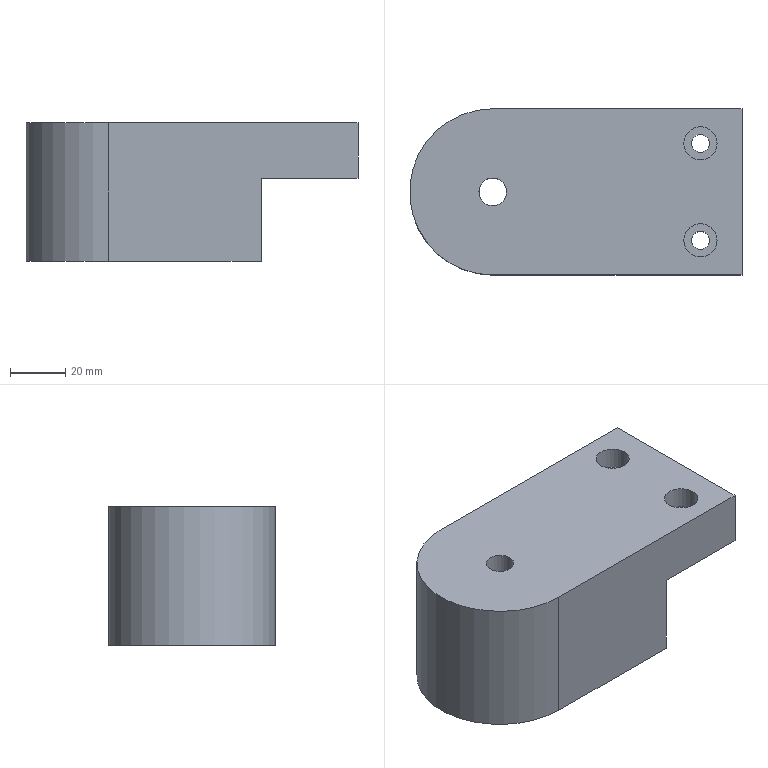Part | NX | 1 solid | 15 faces | box 120 x 60 x 50 mm | volume 271153 mm3 | plane 9 | cylinder 6 | commonest cylinder face diameters 6.5 x2 12 x2 10 x1 60 x1
STEP:
#1=CARTESIAN_POINT('',(25.,-30.,-25.));
#2=VERTEX_POINT('',#1);
#3=CARTESIAN_POINT('',(25.,30.,-25.));
#4=VERTEX_POINT('',#3);
#5=CARTESIAN_POINT('',(25.,-30.,-25.));
#6=DIRECTION('',(0.,1.,0.));
#7=VECTOR('',#6,1.);
#8=LINE('',#5,#7);
#9=EDGE_CURVE('',#2,#4,#8,.T.);
#10=ORIENTED_EDGE('',*,*,#9,.F.);
#11=CARTESIAN_POINT('',(-30.,-30.,-25.));
#12=VERTEX_POINT('',#11);
#13=CARTESIAN_POINT('',(-30.,-30.,-25.));
#14=DIRECTION('',(1.,0.,0.));
#15=VECTOR('',#14,1.);
#16=LINE('',#13,#15);
#17=EDGE_CURVE('',#12,#2,#16,.T.);
#18=ORIENTED_EDGE('',*,*,#17,.F.);
#19=CARTESIAN_POINT('',(-30.,30.,-25.));
#20=VERTEX_POINT('',#19);
#21=CARTESIAN_POINT('',(-30.,0.,-25.));
#22=DIRECTION('',(0.,0.,1.));
#23=DIRECTION('',(0.,1.,0.));
#24=AXIS2_PLACEMENT_3D('',#21,#22,#23);
#25=CIRCLE('',#24,30.);
#26=EDGE_CURVE('',#20,#12,#25,.T.);
#27=ORIENTED_EDGE('',*,*,#26,.F.);
#28=CARTESIAN_POINT('',(25.,30.,-25.));
#29=DIRECTION('',(-1.,0.,0.));
#30=VECTOR('',#29,1.);
#31=LINE('',#28,#30);
#32=EDGE_CURVE('',#4,#20,#31,.T.);
#33=ORIENTED_EDGE('',*,*,#32,.F.);
#34=EDGE_LOOP('',(#10,#18,#27,#33));
#35=FACE_BOUND('',#34,.T.);
#36=CARTESIAN_POINT('',(-35.,0.,-25.));
#37=VERTEX_POINT('',#36);
#38=CARTESIAN_POINT('',(-30.,0.,-25.));
#39=DIRECTION('',(0.,0.,1.));
#40=DIRECTION('',(1.,0.,0.));
#41=AXIS2_PLACEMENT_3D('',#38,#39,#40);
#42=CIRCLE('',#41,5.);
#43=EDGE_CURVE('',#37,#37,#42,.T.);
#44=ORIENTED_EDGE('',*,*,#43,.T.);
#45=EDGE_LOOP('',(#44));
#46=FACE_BOUND('',#45,.T.);
#47=CARTESIAN_POINT('',(0.,0.,-25.));
#48=DIRECTION('',(0.,0.,1.));
#49=DIRECTION('',(1.,0.,0.));
#50=AXIS2_PLACEMENT_3D('',#47,#48,#49);
#51=PLANE('',#50);
#52=ADVANCED_FACE('',(#35,#46),#51,.F.);
#53=CARTESIAN_POINT('',(-30.,-30.,25.));
#54=VERTEX_POINT('',#53);
#55=CARTESIAN_POINT('',(-30.,30.,25.));
#56=VERTEX_POINT('',#55);
#57=CARTESIAN_POINT('',(-30.,0.,25.));
#58=DIRECTION('',(0.,0.,-1.));
#59=DIRECTION('',(0.,-1.,0.));
#60=AXIS2_PLACEMENT_3D('',#57,#58,#59);
#61=CIRCLE('',#60,30.);
#62=EDGE_CURVE('',#54,#56,#61,.T.);
#63=ORIENTED_EDGE('',*,*,#62,.F.);
#64=CARTESIAN_POINT('',(60.,-30.,25.));
#65=VERTEX_POINT('',#64);
#66=CARTESIAN_POINT('',(-30.,-30.,25.));
#67=DIRECTION('',(1.,0.,0.));
#68=VECTOR('',#67,1.);
#69=LINE('',#66,#68);
#70=EDGE_CURVE('',#54,#65,#69,.T.);
#71=ORIENTED_EDGE('',*,*,#70,.T.);
#72=CARTESIAN_POINT('',(60.,30.,25.));
#73=VERTEX_POINT('',#72);
#74=CARTESIAN_POINT('',(60.,-30.,25.));
#75=DIRECTION('',(0.,1.,0.));
#76=VECTOR('',#75,1.);
#77=LINE('',#74,#76);
#78=EDGE_CURVE('',#65,#73,#77,.T.);
#79=ORIENTED_EDGE('',*,*,#78,.T.);
#80=CARTESIAN_POINT('',(60.,30.,25.));
#81=DIRECTION('',(-1.,0.,0.));
#82=VECTOR('',#81,1.);
#83=LINE('',#80,#82);
#84=EDGE_CURVE('',#73,#56,#83,.T.);
#85=ORIENTED_EDGE('',*,*,#84,.T.);
#86=EDGE_LOOP('',(#63,#71,#79,#85));
#87=FACE_BOUND('',#86,.T.);
#88=CARTESIAN_POINT('',(51.,17.5,25.));
#89=VERTEX_POINT('',#88);
#90=CARTESIAN_POINT('',(45.,17.5,25.));
#91=DIRECTION('',(0.,0.,1.));
#92=DIRECTION('',(1.,0.,0.));
#93=AXIS2_PLACEMENT_3D('',#90,#91,#92);
#94=CIRCLE('',#93,6.);
#95=EDGE_CURVE('',#89,#89,#94,.T.);
#96=ORIENTED_EDGE('',*,*,#95,.F.);
#97=EDGE_LOOP('',(#96));
#98=FACE_BOUND('',#97,.T.);
#99=CARTESIAN_POINT('',(51.,-17.5,25.));
#100=VERTEX_POINT('',#99);
#101=CARTESIAN_POINT('',(45.,-17.5,25.));
#102=DIRECTION('',(0.,0.,1.));
#103=DIRECTION('',(1.,0.,0.));
#104=AXIS2_PLACEMENT_3D('',#101,#102,#103);
#105=CIRCLE('',#104,6.);
#106=EDGE_CURVE('',#100,#100,#105,.T.);
#107=ORIENTED_EDGE('',*,*,#106,.F.);
#108=EDGE_LOOP('',(#107));
#109=FACE_BOUND('',#108,.T.);
#110=CARTESIAN_POINT('',(-35.,0.,25.));
#111=VERTEX_POINT('',#110);
#112=CARTESIAN_POINT('',(-30.,0.,25.));
#113=DIRECTION('',(0.,0.,1.));
#114=DIRECTION('',(1.,0.,0.));
#115=AXIS2_PLACEMENT_3D('',#112,#113,#114);
#116=CIRCLE('',#115,5.);
#117=EDGE_CURVE('',#111,#111,#116,.T.);
#118=ORIENTED_EDGE('',*,*,#117,.F.);
#119=EDGE_LOOP('',(#118));
#120=FACE_BOUND('',#119,.T.);
#121=CARTESIAN_POINT('',(0.,0.,25.));
#122=DIRECTION('',(0.,0.,1.));
#123=DIRECTION('',(1.,0.,0.));
#124=AXIS2_PLACEMENT_3D('',#121,#122,#123);
#125=PLANE('',#124);
#126=ADVANCED_FACE('',(#87,#98,#109,#120),#125,.T.);
#127=CARTESIAN_POINT('',(60.,-30.,5.));
#128=VERTEX_POINT('',#127);
#129=CARTESIAN_POINT('',(25.,-30.,5.));
#130=VERTEX_POINT('',#129);
#131=CARTESIAN_POINT('',(60.,-30.,5.));
#132=DIRECTION('',(-1.,0.,0.));
#133=VECTOR('',#132,1.);
#134=LINE('',#131,#133);
#135=EDGE_CURVE('',#128,#130,#134,.T.);
#136=ORIENTED_EDGE('',*,*,#135,.F.);
#137=CARTESIAN_POINT('',(60.,-30.,5.));
#138=DIRECTION('',(0.,0.,1.));
#139=VECTOR('',#138,1.);
#140=LINE('',#137,#139);
#141=EDGE_CURVE('',#128,#65,#140,.T.);
#142=ORIENTED_EDGE('',*,*,#141,.T.);
#143=ORIENTED_EDGE('',*,*,#70,.F.);
#144=CARTESIAN_POINT('',(-30.,-30.,25.));
#145=DIRECTION('',(0.,0.,-1.));
#146=VECTOR('',#145,1.);
#147=LINE('',#144,#146);
#148=EDGE_CURVE('',#54,#12,#147,.T.);
#149=ORIENTED_EDGE('',*,*,#148,.T.);
#150=ORIENTED_EDGE('',*,*,#17,.T.);
#151=CARTESIAN_POINT('',(25.,-30.,-25.));
#152=DIRECTION('',(0.,0.,1.));
#153=VECTOR('',#152,1.);
#154=LINE('',#151,#153);
#155=EDGE_CURVE('',#2,#130,#154,.T.);
#156=ORIENTED_EDGE('',*,*,#155,.T.);
#157=EDGE_LOOP('',(#136,#142,#143,#149,#150,#156));
#158=FACE_OUTER_BOUND('',#157,.T.);
#159=CARTESIAN_POINT('',(-60.,-30.,-25.));
#160=DIRECTION('',(0.,-1.,0.));
#161=DIRECTION('',(0.,0.,-1.));
#162=AXIS2_PLACEMENT_3D('',#159,#160,#161);
#163=PLANE('',#162);
#164=ADVANCED_FACE('',(#158),#163,.T.);
#165=CARTESIAN_POINT('',(60.,30.,5.));
#166=VERTEX_POINT('',#165);
#167=CARTESIAN_POINT('',(60.,-30.,5.));
#168=DIRECTION('',(0.,1.,0.));
#169=VECTOR('',#168,1.);
#170=LINE('',#167,#169);
#171=EDGE_CURVE('',#128,#166,#170,.T.);
#172=ORIENTED_EDGE('',*,*,#171,.T.);
#173=CARTESIAN_POINT('',(60.,30.,5.));
#174=DIRECTION('',(0.,0.,1.));
#175=VECTOR('',#174,1.);
#176=LINE('',#173,#175);
#177=EDGE_CURVE('',#166,#73,#176,.T.);
#178=ORIENTED_EDGE('',*,*,#177,.T.);
#179=ORIENTED_EDGE('',*,*,#78,.F.);
#180=ORIENTED_EDGE('',*,*,#141,.F.);
#181=EDGE_LOOP('',(#172,#178,#179,#180));
#182=FACE_OUTER_BOUND('',#181,.T.);
#183=CARTESIAN_POINT('',(60.,-30.,-25.));
#184=DIRECTION('',(1.,0.,0.));
#185=DIRECTION('',(0.,0.,-1.));
#186=AXIS2_PLACEMENT_3D('',#183,#184,#185);
#187=PLANE('',#186);
#188=ADVANCED_FACE('',(#182),#187,.T.);
#189=CARTESIAN_POINT('',(25.,30.,5.));
#190=VERTEX_POINT('',#189);
#191=CARTESIAN_POINT('',(60.,30.,5.));
#192=DIRECTION('',(-1.,0.,0.));
#193=VECTOR('',#192,1.);
#194=LINE('',#191,#193);
#195=EDGE_CURVE('',#166,#190,#194,.T.);
#196=ORIENTED_EDGE('',*,*,#195,.T.);
#197=CARTESIAN_POINT('',(25.,30.,-25.));
#198=DIRECTION('',(0.,0.,1.));
#199=VECTOR('',#198,1.);
#200=LINE('',#197,#199);
#201=EDGE_CURVE('',#4,#190,#200,.T.);
#202=ORIENTED_EDGE('',*,*,#201,.F.);
#203=ORIENTED_EDGE('',*,*,#32,.T.);
#204=CARTESIAN_POINT('',(-30.,30.,25.));
#205=DIRECTION('',(0.,0.,-1.));
#206=VECTOR('',#205,1.);
#207=LINE('',#204,#206);
#208=EDGE_CURVE('',#56,#20,#207,.T.);
#209=ORIENTED_EDGE('',*,*,#208,.F.);
#210=ORIENTED_EDGE('',*,*,#84,.F.);
#211=ORIENTED_EDGE('',*,*,#177,.F.);
#212=EDGE_LOOP('',(#196,#202,#203,#209,#210,#211));
#213=FACE_OUTER_BOUND('',#212,.T.);
#214=CARTESIAN_POINT('',(60.,30.,-25.));
#215=DIRECTION('',(0.,1.,0.));
#216=DIRECTION('',(0.,0.,1.));
#217=AXIS2_PLACEMENT_3D('',#214,#215,#216);
#218=PLANE('',#217);
#219=ADVANCED_FACE('',(#213),#218,.T.);
#220=ORIENTED_EDGE('',*,*,#62,.T.);
#221=ORIENTED_EDGE('',*,*,#208,.T.);
#222=ORIENTED_EDGE('',*,*,#26,.T.);
#223=ORIENTED_EDGE('',*,*,#148,.F.);
#224=EDGE_LOOP('',(#220,#221,#222,#223));
#225=FACE_OUTER_BOUND('',#224,.T.);
#226=CARTESIAN_POINT('',(-30.,0.,25.231));
#227=DIRECTION('',(0.,0.,-1.));
#228=DIRECTION('',(-1.,0.,0.));
#229=AXIS2_PLACEMENT_3D('',#226,#227,#228);
#230=CYLINDRICAL_SURFACE('',#229,30.);
#231=ADVANCED_FACE('',(#225),#230,.T.);
#232=ORIENTED_EDGE('',*,*,#135,.T.);
#233=CARTESIAN_POINT('',(25.,-30.,5.));
#234=DIRECTION('',(0.,1.,0.));
#235=VECTOR('',#234,1.);
#236=LINE('',#233,#235);
#237=EDGE_CURVE('',#130,#190,#236,.T.);
#238=ORIENTED_EDGE('',*,*,#237,.T.);
#239=ORIENTED_EDGE('',*,*,#195,.F.);
#240=ORIENTED_EDGE('',*,*,#171,.F.);
#241=EDGE_LOOP('',(#232,#238,#239,#240));
#242=FACE_BOUND('',#241,.T.);
#243=CARTESIAN_POINT('',(48.25,17.5,5.));
#244=VERTEX_POINT('',#243);
#245=CARTESIAN_POINT('',(45.,17.5,5.));
#246=DIRECTION('',(0.,0.,1.));
#247=DIRECTION('',(1.,0.,0.));
#248=AXIS2_PLACEMENT_3D('',#245,#246,#247);
#249=CIRCLE('',#248,3.25);
#250=EDGE_CURVE('',#244,#244,#249,.T.);
#251=ORIENTED_EDGE('',*,*,#250,.T.);
#252=EDGE_LOOP('',(#251));
#253=FACE_BOUND('',#252,.T.);
#254=CARTESIAN_POINT('',(48.25,-17.5,5.));
#255=VERTEX_POINT('',#254);
#256=CARTESIAN_POINT('',(45.,-17.5,5.));
#257=DIRECTION('',(0.,0.,1.));
#258=DIRECTION('',(1.,0.,0.));
#259=AXIS2_PLACEMENT_3D('',#256,#257,#258);
#260=CIRCLE('',#259,3.25);
#261=EDGE_CURVE('',#255,#255,#260,.T.);
#262=ORIENTED_EDGE('',*,*,#261,.T.);
#263=EDGE_LOOP('',(#262));
#264=FACE_BOUND('',#263,.T.);
#265=CARTESIAN_POINT('',(0.,0.,5.));
#266=DIRECTION('',(0.,0.,-1.));
#267=DIRECTION('',(-1.,0.,0.));
#268=AXIS2_PLACEMENT_3D('',#265,#266,#267);
#269=PLANE('',#268);
#270=ADVANCED_FACE('',(#242,#253,#264),#269,.T.);
#271=ORIENTED_EDGE('',*,*,#9,.T.);
#272=ORIENTED_EDGE('',*,*,#201,.T.);
#273=ORIENTED_EDGE('',*,*,#237,.F.);
#274=ORIENTED_EDGE('',*,*,#155,.F.);
#275=EDGE_LOOP('',(#271,#272,#273,#274));
#276=FACE_OUTER_BOUND('',#275,.T.);
#277=CARTESIAN_POINT('',(25.,-30.,-25.));
#278=DIRECTION('',(-1.,0.,0.));
#279=DIRECTION('',(0.,0.,1.));
#280=AXIS2_PLACEMENT_3D('',#277,#278,#279);
#281=PLANE('',#280);
#282=ADVANCED_FACE('',(#276),#281,.F.);
#283=CARTESIAN_POINT('',(48.25,17.5,17.));
#284=VERTEX_POINT('',#283);
#285=CARTESIAN_POINT('',(45.,17.5,17.));
#286=DIRECTION('',(0.,0.,1.));
#287=DIRECTION('',(1.,0.,0.));
#288=AXIS2_PLACEMENT_3D('',#285,#286,#287);
#289=CIRCLE('',#288,3.25);
#290=EDGE_CURVE('',#284,#284,#289,.T.);
#291=ORIENTED_EDGE('',*,*,#290,.T.);
#292=EDGE_LOOP('',(#291));
#293=FACE_BOUND('',#292,.T.);
#294=ORIENTED_EDGE('',*,*,#250,.F.);
#295=EDGE_LOOP('',(#294));
#296=FACE_BOUND('',#295,.T.);
#297=CARTESIAN_POINT('',(45.,17.5,25.));
#298=DIRECTION('',(0.,0.,1.));
#299=DIRECTION('',(1.,0.,0.));
#300=AXIS2_PLACEMENT_3D('',#297,#298,#299);
#301=CYLINDRICAL_SURFACE('',#300,3.25);
#302=ADVANCED_FACE('',(#293,#296),#301,.F.);
#303=CARTESIAN_POINT('',(48.25,-17.5,17.));
#304=VERTEX_POINT('',#303);
#305=CARTESIAN_POINT('',(45.,-17.5,17.));
#306=DIRECTION('',(0.,0.,1.));
#307=DIRECTION('',(1.,0.,0.));
#308=AXIS2_PLACEMENT_3D('',#305,#306,#307);
#309=CIRCLE('',#308,3.25);
#310=EDGE_CURVE('',#304,#304,#309,.T.);
#311=ORIENTED_EDGE('',*,*,#310,.T.);
#312=EDGE_LOOP('',(#311));
#313=FACE_BOUND('',#312,.T.);
#314=ORIENTED_EDGE('',*,*,#261,.F.);
#315=EDGE_LOOP('',(#314));
#316=FACE_BOUND('',#315,.T.);
#317=CARTESIAN_POINT('',(45.,-17.5,25.));
#318=DIRECTION('',(0.,0.,1.));
#319=DIRECTION('',(1.,0.,0.));
#320=AXIS2_PLACEMENT_3D('',#317,#318,#319);
#321=CYLINDRICAL_SURFACE('',#320,3.25);
#322=ADVANCED_FACE('',(#313,#316),#321,.F.);
#323=CARTESIAN_POINT('',(51.,17.5,17.));
#324=VERTEX_POINT('',#323);
#325=CARTESIAN_POINT('',(45.,17.5,17.));
#326=DIRECTION('',(0.,0.,1.));
#327=DIRECTION('',(1.,0.,0.));
#328=AXIS2_PLACEMENT_3D('',#325,#326,#327);
#329=CIRCLE('',#328,6.);
#330=EDGE_CURVE('',#324,#324,#329,.T.);
#331=ORIENTED_EDGE('',*,*,#330,.T.);
#332=EDGE_LOOP('',(#331));
#333=FACE_BOUND('',#332,.T.);
#334=ORIENTED_EDGE('',*,*,#290,.F.);
#335=EDGE_LOOP('',(#334));
#336=FACE_BOUND('',#335,.T.);
#337=CARTESIAN_POINT('',(0.,0.,17.));
#338=DIRECTION('',(0.,0.,1.));
#339=DIRECTION('',(1.,0.,0.));
#340=AXIS2_PLACEMENT_3D('',#337,#338,#339);
#341=PLANE('',#340);
#342=ADVANCED_FACE('',(#333,#336),#341,.T.);
#343=CARTESIAN_POINT('',(51.,-17.5,17.));
#344=VERTEX_POINT('',#343);
#345=CARTESIAN_POINT('',(45.,-17.5,17.));
#346=DIRECTION('',(0.,0.,1.));
#347=DIRECTION('',(1.,0.,0.));
#348=AXIS2_PLACEMENT_3D('',#345,#346,#347);
#349=CIRCLE('',#348,6.);
#350=EDGE_CURVE('',#344,#344,#349,.T.);
#351=ORIENTED_EDGE('',*,*,#350,.T.);
#352=EDGE_LOOP('',(#351));
#353=FACE_BOUND('',#352,.T.);
#354=ORIENTED_EDGE('',*,*,#310,.F.);
#355=EDGE_LOOP('',(#354));
#356=FACE_BOUND('',#355,.T.);
#357=CARTESIAN_POINT('',(0.,0.,17.));
#358=DIRECTION('',(0.,0.,1.));
#359=DIRECTION('',(1.,0.,0.));
#360=AXIS2_PLACEMENT_3D('',#357,#358,#359);
#361=PLANE('',#360);
#362=ADVANCED_FACE('',(#353,#356),#361,.T.);
#363=ORIENTED_EDGE('',*,*,#95,.T.);
#364=EDGE_LOOP('',(#363));
#365=FACE_BOUND('',#364,.T.);
#366=ORIENTED_EDGE('',*,*,#330,.F.);
#367=EDGE_LOOP('',(#366));
#368=FACE_BOUND('',#367,.T.);
#369=CARTESIAN_POINT('',(45.,17.5,25.));
#370=DIRECTION('',(0.,0.,1.));
#371=DIRECTION('',(1.,0.,0.));
#372=AXIS2_PLACEMENT_3D('',#369,#370,#371);
#373=CYLINDRICAL_SURFACE('',#372,6.);
#374=ADVANCED_FACE('',(#365,#368),#373,.F.);
#375=ORIENTED_EDGE('',*,*,#106,.T.);
#376=EDGE_LOOP('',(#375));
#377=FACE_BOUND('',#376,.T.);
#378=ORIENTED_EDGE('',*,*,#350,.F.);
#379=EDGE_LOOP('',(#378));
#380=FACE_BOUND('',#379,.T.);
#381=CARTESIAN_POINT('',(45.,-17.5,25.));
#382=DIRECTION('',(0.,0.,1.));
#383=DIRECTION('',(1.,0.,0.));
#384=AXIS2_PLACEMENT_3D('',#381,#382,#383);
#385=CYLINDRICAL_SURFACE('',#384,6.);
#386=ADVANCED_FACE('',(#377,#380),#385,.F.);
#387=ORIENTED_EDGE('',*,*,#43,.F.);
#388=EDGE_LOOP('',(#387));
#389=FACE_BOUND('',#388,.T.);
#390=ORIENTED_EDGE('',*,*,#117,.T.);
#391=EDGE_LOOP('',(#390));
#392=FACE_BOUND('',#391,.T.);
#393=CARTESIAN_POINT('',(-30.,0.,25.));
#394=DIRECTION('',(0.,0.,1.));
#395=DIRECTION('',(1.,0.,0.));
#396=AXIS2_PLACEMENT_3D('',#393,#394,#395);
#397=CYLINDRICAL_SURFACE('',#396,5.);
#398=ADVANCED_FACE('',(#389,#392),#397,.F.);
#399=CLOSED_SHELL('',(#52,#126,#164,#188,#219,#231,#270,#282,#302,#322,#342,#362,#374,#386,#398));
#400=MANIFOLD_SOLID_BREP('',#399);
#401=(LENGTH_UNIT()NAMED_UNIT(*)SI_UNIT(.MILLI.,.METRE.));
#402=UNCERTAINTY_MEASURE_WITH_UNIT(LENGTH_MEASURE(0.00002),#401,'','');
#403=(NAMED_UNIT(*)PLANE_ANGLE_UNIT()SI_UNIT($,.RADIAN.));
#404=PLANE_ANGLE_MEASURE_WITH_UNIT(PLANE_ANGLE_MEASURE(0.01745),#403);
#405=DIMENSIONAL_EXPONENTS(0.,0.,0.,0.,0.,0.,0.);
#406=(CONVERSION_BASED_UNIT('DEGREE',#404)NAMED_UNIT(#405)PLANE_ANGLE_UNIT());
#407=(NAMED_UNIT(*)SI_UNIT($,.STERADIAN.)SOLID_ANGLE_UNIT());
#408=(GEOMETRIC_REPRESENTATION_CONTEXT(3)GLOBAL_UNCERTAINTY_ASSIGNED_CONTEXT((#402))GLOBAL_UNIT_ASSIGNED_CONTEXT((#401,#406,#407))REPRESENTATION_CONTEXT('',''));
#409=ADVANCED_BREP_SHAPE_REPRESENTATION('',(#400),#408);